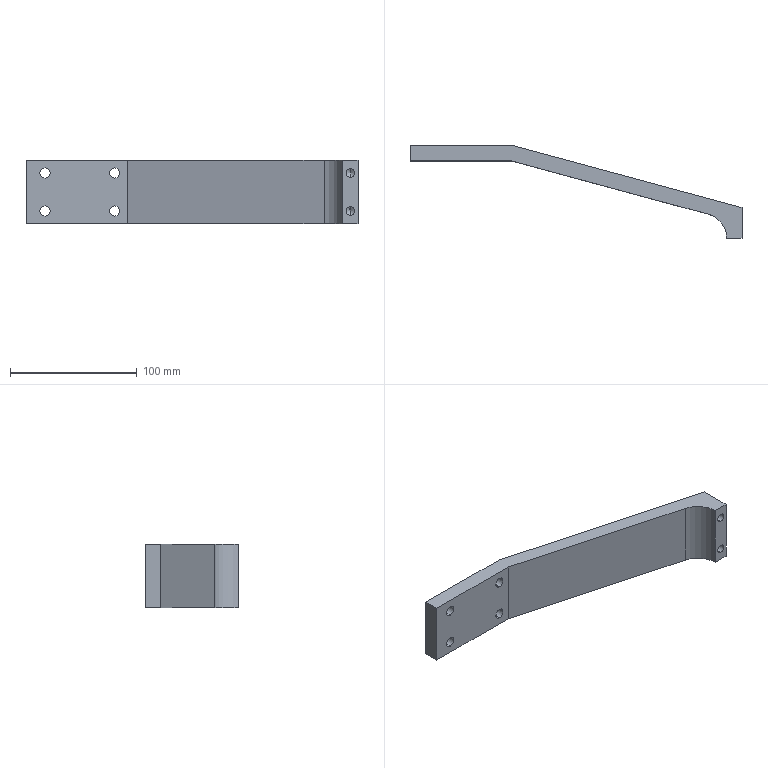Part | SolidWorks | features BaseBody 1 | 1 solid | 26 faces | box 262 x 73 x 50 mm | volume 167970 mm3 | cylinder 13 | plane 9 | cone 4 | commonest cylinder face diameters 8 x8 6.8 x4 40 x1
STEP:
#1=CARTESIAN_POINT('',(-260.,-92.,251.121));
#2=VERTEX_POINT('',#1);
#3=CARTESIAN_POINT('',(-260.,-92.,243.121));
#4=VERTEX_POINT('',#3);
#5=CARTESIAN_POINT('',(-260.,-92.,247.121));
#6=DIRECTION('',(0.,-1.,0.));
#7=DIRECTION('',(0.,0.,1.));
#8=AXIS2_PLACEMENT_3D('',#5,#6,#7);
#9=CIRCLE('',#8,4.);
#10=EDGE_CURVE('',#2,#4,#9,.T.);
#11=ORIENTED_EDGE('',*,*,#10,.T.);
#12=CARTESIAN_POINT('',(-260.,-80.,243.121));
#13=VERTEX_POINT('',#12);
#14=CARTESIAN_POINT('',(-260.,-153.,243.121));
#15=DIRECTION('',(0.,1.,0.));
#16=VECTOR('',#15,1000.);
#17=LINE('',#14,#16);
#18=EDGE_CURVE('',#4,#13,#17,.T.);
#19=ORIENTED_EDGE('',*,*,#18,.T.);
#20=CARTESIAN_POINT('',(-260.,-80.,251.121));
#21=VERTEX_POINT('',#20);
#22=CARTESIAN_POINT('',(-260.,-80.,247.121));
#23=DIRECTION('',(0.,1.,0.));
#24=DIRECTION('',(0.,0.,1.));
#25=AXIS2_PLACEMENT_3D('',#22,#23,#24);
#26=CIRCLE('',#25,4.);
#27=EDGE_CURVE('',#13,#21,#26,.T.);
#28=ORIENTED_EDGE('',*,*,#27,.T.);
#29=CARTESIAN_POINT('',(-260.,-153.,251.121));
#30=DIRECTION('',(0.,1.,0.));
#31=VECTOR('',#30,1000.);
#32=LINE('',#29,#31);
#33=EDGE_CURVE('',#2,#21,#32,.T.);
#34=ORIENTED_EDGE('',*,*,#33,.F.);
#35=EDGE_LOOP('',(#11,#19,#28,#34));
#36=FACE_OUTER_BOUND('',#35,.T.);
#37=CARTESIAN_POINT('',(-260.,-153.,247.121));
#38=DIRECTION('',(0.,1.,0.));
#39=DIRECTION('',(0.,0.,1.));
#40=AXIS2_PLACEMENT_3D('',#37,#38,#39);
#41=CYLINDRICAL_SURFACE('',#40,4.);
#42=ADVANCED_FACE('',(#36),#41,.F.);
#43=CARTESIAN_POINT('',(-260.,-92.,221.121));
#44=VERTEX_POINT('',#43);
#45=CARTESIAN_POINT('',(-260.,-92.,213.121));
#46=VERTEX_POINT('',#45);
#47=CARTESIAN_POINT('',(-260.,-92.,217.121));
#48=DIRECTION('',(0.,-1.,0.));
#49=DIRECTION('',(0.,0.,1.));
#50=AXIS2_PLACEMENT_3D('',#47,#48,#49);
#51=CIRCLE('',#50,4.);
#52=EDGE_CURVE('',#44,#46,#51,.T.);
#53=ORIENTED_EDGE('',*,*,#52,.T.);
#54=CARTESIAN_POINT('',(-260.,-80.,213.121));
#55=VERTEX_POINT('',#54);
#56=CARTESIAN_POINT('',(-260.,-153.,213.121));
#57=DIRECTION('',(0.,1.,0.));
#58=VECTOR('',#57,1000.);
#59=LINE('',#56,#58);
#60=EDGE_CURVE('',#46,#55,#59,.T.);
#61=ORIENTED_EDGE('',*,*,#60,.T.);
#62=CARTESIAN_POINT('',(-260.,-80.,221.121));
#63=VERTEX_POINT('',#62);
#64=CARTESIAN_POINT('',(-260.,-80.,217.121));
#65=DIRECTION('',(0.,1.,0.));
#66=DIRECTION('',(0.,0.,1.));
#67=AXIS2_PLACEMENT_3D('',#64,#65,#66);
#68=CIRCLE('',#67,4.);
#69=EDGE_CURVE('',#55,#63,#68,.T.);
#70=ORIENTED_EDGE('',*,*,#69,.T.);
#71=CARTESIAN_POINT('',(-260.,-153.,221.121));
#72=DIRECTION('',(0.,1.,0.));
#73=VECTOR('',#72,1000.);
#74=LINE('',#71,#73);
#75=EDGE_CURVE('',#44,#63,#74,.T.);
#76=ORIENTED_EDGE('',*,*,#75,.F.);
#77=EDGE_LOOP('',(#53,#61,#70,#76));
#78=FACE_OUTER_BOUND('',#77,.T.);
#79=CARTESIAN_POINT('',(-260.,-153.,217.121));
#80=DIRECTION('',(0.,1.,0.));
#81=DIRECTION('',(0.,0.,1.));
#82=AXIS2_PLACEMENT_3D('',#79,#80,#81);
#83=CYLINDRICAL_SURFACE('',#82,4.);
#84=ADVANCED_FACE('',(#78),#83,.F.);
#85=CARTESIAN_POINT('',(-315.,-92.,221.121));
#86=VERTEX_POINT('',#85);
#87=CARTESIAN_POINT('',(-315.,-92.,213.121));
#88=VERTEX_POINT('',#87);
#89=CARTESIAN_POINT('',(-315.,-92.,217.121));
#90=DIRECTION('',(0.,-1.,0.));
#91=DIRECTION('',(0.,0.,1.));
#92=AXIS2_PLACEMENT_3D('',#89,#90,#91);
#93=CIRCLE('',#92,4.);
#94=EDGE_CURVE('',#86,#88,#93,.T.);
#95=ORIENTED_EDGE('',*,*,#94,.T.);
#96=CARTESIAN_POINT('',(-315.,-80.,213.121));
#97=VERTEX_POINT('',#96);
#98=CARTESIAN_POINT('',(-315.,-153.,213.121));
#99=DIRECTION('',(0.,1.,0.));
#100=VECTOR('',#99,1000.);
#101=LINE('',#98,#100);
#102=EDGE_CURVE('',#88,#97,#101,.T.);
#103=ORIENTED_EDGE('',*,*,#102,.T.);
#104=CARTESIAN_POINT('',(-315.,-80.,221.121));
#105=VERTEX_POINT('',#104);
#106=CARTESIAN_POINT('',(-315.,-80.,217.121));
#107=DIRECTION('',(0.,1.,0.));
#108=DIRECTION('',(0.,0.,1.));
#109=AXIS2_PLACEMENT_3D('',#106,#107,#108);
#110=CIRCLE('',#109,4.);
#111=EDGE_CURVE('',#97,#105,#110,.T.);
#112=ORIENTED_EDGE('',*,*,#111,.T.);
#113=CARTESIAN_POINT('',(-315.,-153.,221.121));
#114=DIRECTION('',(0.,1.,0.));
#115=VECTOR('',#114,1000.);
#116=LINE('',#113,#115);
#117=EDGE_CURVE('',#86,#105,#116,.T.);
#118=ORIENTED_EDGE('',*,*,#117,.F.);
#119=EDGE_LOOP('',(#95,#103,#112,#118));
#120=FACE_OUTER_BOUND('',#119,.T.);
#121=CARTESIAN_POINT('',(-315.,-153.,217.121));
#122=DIRECTION('',(0.,1.,0.));
#123=DIRECTION('',(0.,0.,1.));
#124=AXIS2_PLACEMENT_3D('',#121,#122,#123);
#125=CYLINDRICAL_SURFACE('',#124,4.);
#126=ADVANCED_FACE('',(#120),#125,.F.);
#127=CARTESIAN_POINT('',(-315.,-92.,251.121));
#128=VERTEX_POINT('',#127);
#129=CARTESIAN_POINT('',(-315.,-92.,243.121));
#130=VERTEX_POINT('',#129);
#131=CARTESIAN_POINT('',(-315.,-92.,247.121));
#132=DIRECTION('',(0.,-1.,0.));
#133=DIRECTION('',(0.,0.,1.));
#134=AXIS2_PLACEMENT_3D('',#131,#132,#133);
#135=CIRCLE('',#134,4.);
#136=EDGE_CURVE('',#128,#130,#135,.T.);
#137=ORIENTED_EDGE('',*,*,#136,.T.);
#138=CARTESIAN_POINT('',(-315.,-80.,243.121));
#139=VERTEX_POINT('',#138);
#140=CARTESIAN_POINT('',(-315.,-153.,243.121));
#141=DIRECTION('',(0.,1.,0.));
#142=VECTOR('',#141,1000.);
#143=LINE('',#140,#142);
#144=EDGE_CURVE('',#130,#139,#143,.T.);
#145=ORIENTED_EDGE('',*,*,#144,.T.);
#146=CARTESIAN_POINT('',(-315.,-80.,251.121));
#147=VERTEX_POINT('',#146);
#148=CARTESIAN_POINT('',(-315.,-80.,247.121));
#149=DIRECTION('',(0.,1.,0.));
#150=DIRECTION('',(0.,0.,1.));
#151=AXIS2_PLACEMENT_3D('',#148,#149,#150);
#152=CIRCLE('',#151,4.);
#153=EDGE_CURVE('',#139,#147,#152,.T.);
#154=ORIENTED_EDGE('',*,*,#153,.T.);
#155=CARTESIAN_POINT('',(-315.,-153.,251.121));
#156=DIRECTION('',(0.,1.,0.));
#157=VECTOR('',#156,1000.);
#158=LINE('',#155,#157);
#159=EDGE_CURVE('',#128,#147,#158,.T.);
#160=ORIENTED_EDGE('',*,*,#159,.F.);
#161=EDGE_LOOP('',(#137,#145,#154,#160));
#162=FACE_OUTER_BOUND('',#161,.T.);
#163=CARTESIAN_POINT('',(-315.,-153.,247.121));
#164=DIRECTION('',(0.,1.,0.));
#165=DIRECTION('',(0.,0.,1.));
#166=AXIS2_PLACEMENT_3D('',#163,#164,#165);
#167=CYLINDRICAL_SURFACE('',#166,4.);
#168=ADVANCED_FACE('',(#162),#167,.F.);
#169=CARTESIAN_POINT('',(-74.,-140.,220.521));
#170=VERTEX_POINT('',#169);
#171=CARTESIAN_POINT('',(-74.,-140.,213.721));
#172=VERTEX_POINT('',#171);
#173=CARTESIAN_POINT('',(-74.,-140.,217.121));
#174=DIRECTION('',(0.,-1.,0.));
#175=DIRECTION('',(0.,0.,-1.));
#176=AXIS2_PLACEMENT_3D('',#173,#174,#175);
#177=CIRCLE('',#176,3.4);
#178=EDGE_CURVE('',#170,#172,#177,.T.);
#179=ORIENTED_EDGE('',*,*,#178,.F.);
#180=CARTESIAN_POINT('',(-74.,-153.,220.521));
#181=VERTEX_POINT('',#180);
#182=CARTESIAN_POINT('',(-74.,-153.,220.521));
#183=DIRECTION('',(0.,-1.,0.));
#184=VECTOR('',#183,1000.);
#185=LINE('',#182,#184);
#186=EDGE_CURVE('',#170,#181,#185,.T.);
#187=ORIENTED_EDGE('',*,*,#186,.T.);
#188=CARTESIAN_POINT('',(-74.,-153.,213.721));
#189=VERTEX_POINT('',#188);
#190=CARTESIAN_POINT('',(-74.,-153.,217.121));
#191=DIRECTION('',(0.,-1.,0.));
#192=DIRECTION('',(0.,0.,-1.));
#193=AXIS2_PLACEMENT_3D('',#190,#191,#192);
#194=CIRCLE('',#193,3.4);
#195=EDGE_CURVE('',#181,#189,#194,.T.);
#196=ORIENTED_EDGE('',*,*,#195,.T.);
#197=CARTESIAN_POINT('',(-74.,-153.,213.721));
#198=DIRECTION('',(0.,-1.,0.));
#199=VECTOR('',#198,1000.);
#200=LINE('',#197,#199);
#201=EDGE_CURVE('',#172,#189,#200,.T.);
#202=ORIENTED_EDGE('',*,*,#201,.F.);
#203=EDGE_LOOP('',(#179,#187,#196,#202));
#204=FACE_OUTER_BOUND('',#203,.T.);
#205=CARTESIAN_POINT('',(-74.,-153.,217.121));
#206=DIRECTION('',(0.,-1.,0.));
#207=DIRECTION('',(0.,0.,-1.));
#208=AXIS2_PLACEMENT_3D('',#205,#206,#207);
#209=CYLINDRICAL_SURFACE('',#208,3.4);
#210=ADVANCED_FACE('',(#204),#209,.F.);
#211=CARTESIAN_POINT('',(-74.,-140.,250.521));
#212=VERTEX_POINT('',#211);
#213=CARTESIAN_POINT('',(-74.,-140.,243.721));
#214=VERTEX_POINT('',#213);
#215=CARTESIAN_POINT('',(-74.,-140.,247.121));
#216=DIRECTION('',(0.,-1.,0.));
#217=DIRECTION('',(0.,0.,-1.));
#218=AXIS2_PLACEMENT_3D('',#215,#216,#217);
#219=CIRCLE('',#218,3.4);
#220=EDGE_CURVE('',#212,#214,#219,.T.);
#221=ORIENTED_EDGE('',*,*,#220,.F.);
#222=CARTESIAN_POINT('',(-74.,-153.,250.521));
#223=VERTEX_POINT('',#222);
#224=CARTESIAN_POINT('',(-74.,-153.,250.521));
#225=DIRECTION('',(0.,-1.,0.));
#226=VECTOR('',#225,1000.);
#227=LINE('',#224,#226);
#228=EDGE_CURVE('',#212,#223,#227,.T.);
#229=ORIENTED_EDGE('',*,*,#228,.T.);
#230=CARTESIAN_POINT('',(-74.,-153.,243.721));
#231=VERTEX_POINT('',#230);
#232=CARTESIAN_POINT('',(-74.,-153.,247.121));
#233=DIRECTION('',(0.,-1.,0.));
#234=DIRECTION('',(0.,0.,-1.));
#235=AXIS2_PLACEMENT_3D('',#232,#233,#234);
#236=CIRCLE('',#235,3.4);
#237=EDGE_CURVE('',#223,#231,#236,.T.);
#238=ORIENTED_EDGE('',*,*,#237,.T.);
#239=CARTESIAN_POINT('',(-74.,-153.,243.721));
#240=DIRECTION('',(0.,-1.,0.));
#241=VECTOR('',#240,1000.);
#242=LINE('',#239,#241);
#243=EDGE_CURVE('',#214,#231,#242,.T.);
#244=ORIENTED_EDGE('',*,*,#243,.F.);
#245=EDGE_LOOP('',(#221,#229,#238,#244));
#246=FACE_OUTER_BOUND('',#245,.T.);
#247=CARTESIAN_POINT('',(-74.,-153.,247.121));
#248=DIRECTION('',(0.,-1.,0.));
#249=DIRECTION('',(0.,0.,-1.));
#250=AXIS2_PLACEMENT_3D('',#247,#248,#249);
#251=CYLINDRICAL_SURFACE('',#250,3.4);
#252=ADVANCED_FACE('',(#246),#251,.F.);
#253=CARTESIAN_POINT('',(-74.,-137.957,217.121));
#254=VERTEX_POINT('',#253);
#255=CARTESIAN_POINT('',(-74.,-140.,213.721));
#256=DIRECTION('',(0.,-0.515,-0.8572));
#257=VECTOR('',#256,1000.);
#258=LINE('',#255,#257);
#259=EDGE_CURVE('',#254,#172,#258,.T.);
#260=ORIENTED_EDGE('',*,*,#259,.F.);
#261=CARTESIAN_POINT('',(-74.,-140.,220.521));
#262=DIRECTION('',(0.,-0.515,0.8572));
#263=VECTOR('',#262,1000.);
#264=LINE('',#261,#263);
#265=EDGE_CURVE('',#254,#170,#264,.T.);
#266=ORIENTED_EDGE('',*,*,#265,.T.);
#267=ORIENTED_EDGE('',*,*,#178,.T.);
#268=EDGE_LOOP('',(#260,#266,#267));
#269=FACE_OUTER_BOUND('',#268,.T.);
#270=CARTESIAN_POINT('',(-74.,-140.,217.121));
#271=DIRECTION('',(0.,-1.,0.));
#272=DIRECTION('',(0.,0.,-1.));
#273=AXIS2_PLACEMENT_3D('',#270,#271,#272);
#274=CONICAL_SURFACE('',#273,3.4,1.03);
#275=ADVANCED_FACE('',(#269),#274,.F.);
#276=CARTESIAN_POINT('',(-74.,-137.957,247.121));
#277=VERTEX_POINT('',#276);
#278=CARTESIAN_POINT('',(-74.,-140.,243.721));
#279=DIRECTION('',(0.,-0.515,-0.8572));
#280=VECTOR('',#279,1000.);
#281=LINE('',#278,#280);
#282=EDGE_CURVE('',#277,#214,#281,.T.);
#283=ORIENTED_EDGE('',*,*,#282,.F.);
#284=CARTESIAN_POINT('',(-74.,-140.,250.521));
#285=DIRECTION('',(0.,-0.515,0.8572));
#286=VECTOR('',#285,1000.);
#287=LINE('',#284,#286);
#288=EDGE_CURVE('',#277,#212,#287,.T.);
#289=ORIENTED_EDGE('',*,*,#288,.T.);
#290=ORIENTED_EDGE('',*,*,#220,.T.);
#291=EDGE_LOOP('',(#283,#289,#290));
#292=FACE_OUTER_BOUND('',#291,.T.);
#293=CARTESIAN_POINT('',(-74.,-140.,247.121));
#294=DIRECTION('',(0.,-1.,0.));
#295=DIRECTION('',(0.,0.,-1.));
#296=AXIS2_PLACEMENT_3D('',#293,#294,#295);
#297=CONICAL_SURFACE('',#296,3.4,1.03);
#298=ADVANCED_FACE('',(#292),#297,.F.);
#299=CARTESIAN_POINT('',(-248.405,-80.,257.121));
#300=VERTEX_POINT('',#299);
#301=CARTESIAN_POINT('',(-248.405,-80.,207.121));
#302=VERTEX_POINT('',#301);
#303=CARTESIAN_POINT('',(-248.405,-80.,257.121));
#304=DIRECTION('',(0.,0.,-1.));
#305=VECTOR('',#304,1000.);
#306=LINE('',#303,#305);
#307=EDGE_CURVE('',#300,#302,#306,.T.);
#308=ORIENTED_EDGE('',*,*,#307,.F.);
#309=CARTESIAN_POINT('',(-68.,-128.816,257.121));
#310=VERTEX_POINT('',#309);
#311=CARTESIAN_POINT('',(-68.,-128.816,257.121));
#312=DIRECTION('',(-0.9653,0.2612,0.));
#313=VECTOR('',#312,1000.);
#314=LINE('',#311,#313);
#315=EDGE_CURVE('',#310,#300,#314,.T.);
#316=ORIENTED_EDGE('',*,*,#315,.F.);
#317=CARTESIAN_POINT('',(-68.,-128.816,207.121));
#318=VERTEX_POINT('',#317);
#319=CARTESIAN_POINT('',(-68.,-128.816,257.121));
#320=DIRECTION('',(0.,0.,1.));
#321=VECTOR('',#320,1000.);
#322=LINE('',#319,#321);
#323=EDGE_CURVE('',#318,#310,#322,.T.);
#324=ORIENTED_EDGE('',*,*,#323,.F.);
#325=CARTESIAN_POINT('',(-68.,-128.816,207.121));
#326=DIRECTION('',(0.9653,-0.2612,0.));
#327=VECTOR('',#326,1000.);
#328=LINE('',#325,#327);
#329=EDGE_CURVE('',#302,#318,#328,.T.);
#330=ORIENTED_EDGE('',*,*,#329,.F.);
#331=EDGE_LOOP('',(#308,#316,#324,#330));
#332=FACE_OUTER_BOUND('',#331,.T.);
#333=CARTESIAN_POINT('',(-68.,-128.816,257.121));
#334=DIRECTION('',(-0.2612,-0.9653,0.));
#335=DIRECTION('',(0.9653,-0.2612,0.));
#336=AXIS2_PLACEMENT_3D('',#333,#334,#335);
#337=PLANE('',#336);
#338=ADVANCED_FACE('',(#332),#337,.F.);
#339=CARTESIAN_POINT('',(-94.774,-134.002,207.121));
#340=VERTEX_POINT('',#339);
#341=CARTESIAN_POINT('',(-80.,-153.,207.121));
#342=VERTEX_POINT('',#341);
#343=CARTESIAN_POINT('',(-99.998,-153.308,207.121));
#344=DIRECTION('',(0.,0.,-1.));
#345=DIRECTION('',(1.,0.,0.));
#346=AXIS2_PLACEMENT_3D('',#343,#344,#345);
#347=CIRCLE('',#346,20.);
#348=EDGE_CURVE('',#340,#342,#347,.T.);
#349=ORIENTED_EDGE('',*,*,#348,.F.);
#350=CARTESIAN_POINT('',(-250.,-92.,207.121));
#351=VERTEX_POINT('',#350);
#352=CARTESIAN_POINT('',(-250.,-92.,207.121));
#353=DIRECTION('',(0.9653,-0.2612,0.));
#354=VECTOR('',#353,1000.);
#355=LINE('',#352,#354);
#356=EDGE_CURVE('',#351,#340,#355,.T.);
#357=ORIENTED_EDGE('',*,*,#356,.F.);
#358=CARTESIAN_POINT('',(-330.,-92.,207.121));
#359=VERTEX_POINT('',#358);
#360=CARTESIAN_POINT('',(-68.,-92.,207.121));
#361=DIRECTION('',(1.,0.,0.));
#362=VECTOR('',#361,1000.);
#363=LINE('',#360,#362);
#364=EDGE_CURVE('',#359,#351,#363,.T.);
#365=ORIENTED_EDGE('',*,*,#364,.F.);
#366=CARTESIAN_POINT('',(-330.,-80.,207.121));
#367=VERTEX_POINT('',#366);
#368=CARTESIAN_POINT('',(-330.,-108.6,207.121));
#369=DIRECTION('',(0.,-1.,0.));
#370=VECTOR('',#369,1000.);
#371=LINE('',#368,#370);
#372=EDGE_CURVE('',#367,#359,#371,.T.);
#373=ORIENTED_EDGE('',*,*,#372,.F.);
#374=CARTESIAN_POINT('',(-68.,-80.,207.121));
#375=DIRECTION('',(-1.,0.,0.));
#376=VECTOR('',#375,1000.);
#377=LINE('',#374,#376);
#378=EDGE_CURVE('',#302,#367,#377,.T.);
#379=ORIENTED_EDGE('',*,*,#378,.F.);
#380=ORIENTED_EDGE('',*,*,#329,.T.);
#381=CARTESIAN_POINT('',(-68.,-153.,207.121));
#382=VERTEX_POINT('',#381);
#383=CARTESIAN_POINT('',(-68.,-108.6,207.121));
#384=DIRECTION('',(0.,1.,0.));
#385=VECTOR('',#384,1000.);
#386=LINE('',#383,#385);
#387=EDGE_CURVE('',#382,#318,#386,.T.);
#388=ORIENTED_EDGE('',*,*,#387,.F.);
#389=CARTESIAN_POINT('',(-68.,-153.,207.121));
#390=DIRECTION('',(1.,0.,0.));
#391=VECTOR('',#390,1000.);
#392=LINE('',#389,#391);
#393=EDGE_CURVE('',#342,#382,#392,.T.);
#394=ORIENTED_EDGE('',*,*,#393,.F.);
#395=EDGE_LOOP('',(#349,#357,#365,#373,#379,#380,#388,#394));
#396=FACE_OUTER_BOUND('',#395,.T.);
#397=CARTESIAN_POINT('',(-68.,-108.6,207.121));
#398=DIRECTION('',(0.,0.,1.));
#399=DIRECTION('',(1.,0.,0.));
#400=AXIS2_PLACEMENT_3D('',#397,#398,#399);
#401=PLANE('',#400);
#402=ADVANCED_FACE('',(#396),#401,.F.);
#403=CARTESIAN_POINT('',(-330.,-80.,257.121));
#404=VERTEX_POINT('',#403);
#405=CARTESIAN_POINT('',(-330.,-80.,257.121));
#406=DIRECTION('',(0.,0.,-1.));
#407=VECTOR('',#406,1000.);
#408=LINE('',#405,#407);
#409=EDGE_CURVE('',#404,#367,#408,.T.);
#410=ORIENTED_EDGE('',*,*,#409,.F.);
#411=CARTESIAN_POINT('',(-248.405,-80.,257.121));
#412=DIRECTION('',(-1.,0.,0.));
#413=VECTOR('',#412,1000.);
#414=LINE('',#411,#413);
#415=EDGE_CURVE('',#300,#404,#414,.T.);
#416=ORIENTED_EDGE('',*,*,#415,.F.);
#417=ORIENTED_EDGE('',*,*,#307,.T.);
#418=ORIENTED_EDGE('',*,*,#378,.T.);
#419=EDGE_LOOP('',(#410,#416,#417,#418));
#420=FACE_OUTER_BOUND('',#419,.T.);
#421=CARTESIAN_POINT('',(-260.,-80.,247.121));
#422=DIRECTION('',(0.,1.,0.));
#423=DIRECTION('',(0.,0.,1.));
#424=AXIS2_PLACEMENT_3D('',#421,#422,#423);
#425=CIRCLE('',#424,4.);
#426=EDGE_CURVE('',#21,#13,#425,.T.);
#427=ORIENTED_EDGE('',*,*,#426,.F.);
#428=ORIENTED_EDGE('',*,*,#27,.F.);
#429=EDGE_LOOP('',(#427,#428));
#430=FACE_BOUND('',#429,.T.);
#431=CARTESIAN_POINT('',(-260.,-80.,217.121));
#432=DIRECTION('',(0.,1.,0.));
#433=DIRECTION('',(0.,0.,1.));
#434=AXIS2_PLACEMENT_3D('',#431,#432,#433);
#435=CIRCLE('',#434,4.);
#436=EDGE_CURVE('',#63,#55,#435,.T.);
#437=ORIENTED_EDGE('',*,*,#436,.F.);
#438=ORIENTED_EDGE('',*,*,#69,.F.);
#439=EDGE_LOOP('',(#437,#438));
#440=FACE_BOUND('',#439,.T.);
#441=CARTESIAN_POINT('',(-315.,-80.,217.121));
#442=DIRECTION('',(0.,1.,0.));
#443=DIRECTION('',(0.,0.,1.));
#444=AXIS2_PLACEMENT_3D('',#441,#442,#443);
#445=CIRCLE('',#444,4.);
#446=EDGE_CURVE('',#105,#97,#445,.T.);
#447=ORIENTED_EDGE('',*,*,#446,.F.);
#448=ORIENTED_EDGE('',*,*,#111,.F.);
#449=EDGE_LOOP('',(#447,#448));
#450=FACE_BOUND('',#449,.T.);
#451=CARTESIAN_POINT('',(-315.,-80.,247.121));
#452=DIRECTION('',(0.,1.,0.));
#453=DIRECTION('',(0.,0.,1.));
#454=AXIS2_PLACEMENT_3D('',#451,#452,#453);
#455=CIRCLE('',#454,4.);
#456=EDGE_CURVE('',#147,#139,#455,.T.);
#457=ORIENTED_EDGE('',*,*,#456,.F.);
#458=ORIENTED_EDGE('',*,*,#153,.F.);
#459=EDGE_LOOP('',(#457,#458));
#460=FACE_BOUND('',#459,.T.);
#461=CARTESIAN_POINT('',(-248.405,-80.,257.121));
#462=DIRECTION('',(0.,-1.,0.));
#463=DIRECTION('',(0.,0.,-1.));
#464=AXIS2_PLACEMENT_3D('',#461,#462,#463);
#465=PLANE('',#464);
#466=ADVANCED_FACE('',(#420,#430,#440,#450,#460),#465,.F.);
#467=CARTESIAN_POINT('',(-250.,-92.,257.121));
#468=VERTEX_POINT('',#467);
#469=CARTESIAN_POINT('',(-94.774,-134.002,257.121));
#470=VERTEX_POINT('',#469);
#471=CARTESIAN_POINT('',(-250.,-92.,257.121));
#472=DIRECTION('',(0.9653,-0.2612,0.));
#473=VECTOR('',#472,1000.);
#474=LINE('',#471,#473);
#475=EDGE_CURVE('',#468,#470,#474,.T.);
#476=ORIENTED_EDGE('',*,*,#475,.T.);
#477=CARTESIAN_POINT('',(-80.,-153.,257.121));
#478=VERTEX_POINT('',#477);
#479=CARTESIAN_POINT('',(-99.998,-153.308,257.121));
#480=DIRECTION('',(0.,0.,-1.));
#481=DIRECTION('',(1.,0.,0.));
#482=AXIS2_PLACEMENT_3D('',#479,#480,#481);
#483=CIRCLE('',#482,20.);
#484=EDGE_CURVE('',#470,#478,#483,.T.);
#485=ORIENTED_EDGE('',*,*,#484,.T.);
#486=CARTESIAN_POINT('',(-68.,-153.,257.121));
#487=VERTEX_POINT('',#486);
#488=CARTESIAN_POINT('',(-68.,-153.,257.121));
#489=DIRECTION('',(1.,0.,0.));
#490=VECTOR('',#489,1000.);
#491=LINE('',#488,#490);
#492=EDGE_CURVE('',#478,#487,#491,.T.);
#493=ORIENTED_EDGE('',*,*,#492,.T.);
#494=CARTESIAN_POINT('',(-68.,-108.6,257.121));
#495=DIRECTION('',(0.,1.,0.));
#496=VECTOR('',#495,1000.);
#497=LINE('',#494,#496);
#498=EDGE_CURVE('',#487,#310,#497,.T.);
#499=ORIENTED_EDGE('',*,*,#498,.T.);
#500=ORIENTED_EDGE('',*,*,#315,.T.);
#501=ORIENTED_EDGE('',*,*,#415,.T.);
#502=CARTESIAN_POINT('',(-330.,-92.,257.121));
#503=VERTEX_POINT('',#502);
#504=CARTESIAN_POINT('',(-330.,-108.6,257.121));
#505=DIRECTION('',(0.,-1.,0.));
#506=VECTOR('',#505,1000.);
#507=LINE('',#504,#506);
#508=EDGE_CURVE('',#404,#503,#507,.T.);
#509=ORIENTED_EDGE('',*,*,#508,.T.);
#510=CARTESIAN_POINT('',(-68.,-92.,257.121));
#511=DIRECTION('',(1.,0.,0.));
#512=VECTOR('',#511,1000.);
#513=LINE('',#510,#512);
#514=EDGE_CURVE('',#503,#468,#513,.T.);
#515=ORIENTED_EDGE('',*,*,#514,.T.);
#516=EDGE_LOOP('',(#476,#485,#493,#499,#500,#501,#509,#515));
#517=FACE_OUTER_BOUND('',#516,.T.);
#518=CARTESIAN_POINT('',(-68.,-108.6,257.121));
#519=DIRECTION('',(0.,0.,1.));
#520=DIRECTION('',(1.,0.,0.));
#521=AXIS2_PLACEMENT_3D('',#518,#519,#520);
#522=PLANE('',#521);
#523=ADVANCED_FACE('',(#517),#522,.T.);
#524=ORIENTED_EDGE('',*,*,#323,.T.);
#525=ORIENTED_EDGE('',*,*,#498,.F.);
#526=CARTESIAN_POINT('',(-68.,-153.,257.121));
#527=DIRECTION('',(0.,0.,1.));
#528=VECTOR('',#527,1000.);
#529=LINE('',#526,#528);
#530=EDGE_CURVE('',#382,#487,#529,.T.);
#531=ORIENTED_EDGE('',*,*,#530,.F.);
#532=ORIENTED_EDGE('',*,*,#387,.T.);
#533=EDGE_LOOP('',(#524,#525,#531,#532));
#534=FACE_OUTER_BOUND('',#533,.T.);
#535=CARTESIAN_POINT('',(-68.,-153.,257.121));
#536=DIRECTION('',(-1.,0.,0.));
#537=DIRECTION('',(0.,0.,1.));
#538=AXIS2_PLACEMENT_3D('',#535,#536,#537);
#539=PLANE('',#538);
#540=ADVANCED_FACE('',(#534),#539,.F.);
#541=ORIENTED_EDGE('',*,*,#530,.T.);
#542=ORIENTED_EDGE('',*,*,#492,.F.);
#543=CARTESIAN_POINT('',(-80.,-153.,257.121));
#544=DIRECTION('',(0.,0.,1.));
#545=VECTOR('',#544,1000.);
#546=LINE('',#543,#545);
#547=EDGE_CURVE('',#342,#478,#546,.T.);
#548=ORIENTED_EDGE('',*,*,#547,.F.);
#549=ORIENTED_EDGE('',*,*,#393,.T.);
#550=EDGE_LOOP('',(#541,#542,#548,#549));
#551=FACE_OUTER_BOUND('',#550,.T.);
#552=CARTESIAN_POINT('',(-74.,-153.,217.121));
#553=DIRECTION('',(0.,-1.,0.));
#554=DIRECTION('',(0.,0.,-1.));
#555=AXIS2_PLACEMENT_3D('',#552,#553,#554);
#556=CIRCLE('',#555,3.4);
#557=EDGE_CURVE('',#189,#181,#556,.T.);
#558=ORIENTED_EDGE('',*,*,#557,.F.);
#559=ORIENTED_EDGE('',*,*,#195,.F.);
#560=EDGE_LOOP('',(#558,#559));
#561=FACE_BOUND('',#560,.T.);
#562=CARTESIAN_POINT('',(-74.,-153.,247.121));
#563=DIRECTION('',(0.,-1.,0.));
#564=DIRECTION('',(0.,0.,-1.));
#565=AXIS2_PLACEMENT_3D('',#562,#563,#564);
#566=CIRCLE('',#565,3.4);
#567=EDGE_CURVE('',#231,#223,#566,.T.);
#568=ORIENTED_EDGE('',*,*,#567,.F.);
#569=ORIENTED_EDGE('',*,*,#237,.F.);
#570=EDGE_LOOP('',(#568,#569));
#571=FACE_BOUND('',#570,.T.);
#572=CARTESIAN_POINT('',(-80.,-153.,257.121));
#573=DIRECTION('',(0.,1.,0.));
#574=DIRECTION('',(0.,0.,1.));
#575=AXIS2_PLACEMENT_3D('',#572,#573,#574);
#576=PLANE('',#575);
#577=ADVANCED_FACE('',(#551,#561,#571),#576,.F.);
#578=CARTESIAN_POINT('',(-94.774,-134.002,257.121));
#579=DIRECTION('',(0.,0.,1.));
#580=VECTOR('',#579,1000.);
#581=LINE('',#578,#580);
#582=EDGE_CURVE('',#340,#470,#581,.T.);
#583=ORIENTED_EDGE('',*,*,#582,.F.);
#584=ORIENTED_EDGE('',*,*,#348,.T.);
#585=ORIENTED_EDGE('',*,*,#547,.T.);
#586=ORIENTED_EDGE('',*,*,#484,.F.);
#587=EDGE_LOOP('',(#583,#584,#585,#586));
#588=FACE_OUTER_BOUND('',#587,.T.);
#589=CARTESIAN_POINT('',(-99.998,-153.308,257.121));
#590=DIRECTION('',(0.,0.,1.));
#591=DIRECTION('',(1.,0.,0.));
#592=AXIS2_PLACEMENT_3D('',#589,#590,#591);
#593=CYLINDRICAL_SURFACE('',#592,20.);
#594=ADVANCED_FACE('',(#588),#593,.F.);
#595=ORIENTED_EDGE('',*,*,#582,.T.);
#596=ORIENTED_EDGE('',*,*,#475,.F.);
#597=CARTESIAN_POINT('',(-250.,-92.,257.121));
#598=DIRECTION('',(0.,0.,1.));
#599=VECTOR('',#598,1000.);
#600=LINE('',#597,#599);
#601=EDGE_CURVE('',#351,#468,#600,.T.);
#602=ORIENTED_EDGE('',*,*,#601,.F.);
#603=ORIENTED_EDGE('',*,*,#356,.T.);
#604=EDGE_LOOP('',(#595,#596,#602,#603));
#605=FACE_OUTER_BOUND('',#604,.T.);
#606=CARTESIAN_POINT('',(-80.,-138.,257.121));
#607=DIRECTION('',(0.2612,0.9653,0.));
#608=DIRECTION('',(-0.9653,0.2612,0.));
#609=AXIS2_PLACEMENT_3D('',#606,#607,#608);
#610=PLANE('',#609);
#611=ADVANCED_FACE('',(#605),#610,.F.);
#612=ORIENTED_EDGE('',*,*,#601,.T.);
#613=ORIENTED_EDGE('',*,*,#514,.F.);
#614=CARTESIAN_POINT('',(-330.,-92.,257.121));
#615=DIRECTION('',(0.,0.,1.));
#616=VECTOR('',#615,1000.);
#617=LINE('',#614,#616);
#618=EDGE_CURVE('',#359,#503,#617,.T.);
#619=ORIENTED_EDGE('',*,*,#618,.F.);
#620=ORIENTED_EDGE('',*,*,#364,.T.);
#621=EDGE_LOOP('',(#612,#613,#619,#620));
#622=FACE_OUTER_BOUND('',#621,.T.);
#623=ORIENTED_EDGE('',*,*,#10,.F.);
#624=CARTESIAN_POINT('',(-260.,-92.,247.121));
#625=DIRECTION('',(0.,-1.,0.));
#626=DIRECTION('',(0.,0.,1.));
#627=AXIS2_PLACEMENT_3D('',#624,#625,#626);
#628=CIRCLE('',#627,4.);
#629=EDGE_CURVE('',#4,#2,#628,.T.);
#630=ORIENTED_EDGE('',*,*,#629,.F.);
#631=EDGE_LOOP('',(#623,#630));
#632=FACE_BOUND('',#631,.T.);
#633=ORIENTED_EDGE('',*,*,#52,.F.);
#634=CARTESIAN_POINT('',(-260.,-92.,217.121));
#635=DIRECTION('',(0.,-1.,0.));
#636=DIRECTION('',(0.,0.,1.));
#637=AXIS2_PLACEMENT_3D('',#634,#635,#636);
#638=CIRCLE('',#637,4.);
#639=EDGE_CURVE('',#46,#44,#638,.T.);
#640=ORIENTED_EDGE('',*,*,#639,.F.);
#641=EDGE_LOOP('',(#633,#640));
#642=FACE_BOUND('',#641,.T.);
#643=ORIENTED_EDGE('',*,*,#94,.F.);
#644=CARTESIAN_POINT('',(-315.,-92.,217.121));
#645=DIRECTION('',(0.,-1.,0.));
#646=DIRECTION('',(0.,0.,1.));
#647=AXIS2_PLACEMENT_3D('',#644,#645,#646);
#648=CIRCLE('',#647,4.);
#649=EDGE_CURVE('',#88,#86,#648,.T.);
#650=ORIENTED_EDGE('',*,*,#649,.F.);
#651=EDGE_LOOP('',(#643,#650));
#652=FACE_BOUND('',#651,.T.);
#653=ORIENTED_EDGE('',*,*,#136,.F.);
#654=CARTESIAN_POINT('',(-315.,-92.,247.121));
#655=DIRECTION('',(0.,-1.,0.));
#656=DIRECTION('',(0.,0.,1.));
#657=AXIS2_PLACEMENT_3D('',#654,#655,#656);
#658=CIRCLE('',#657,4.);
#659=EDGE_CURVE('',#130,#128,#658,.T.);
#660=ORIENTED_EDGE('',*,*,#659,.F.);
#661=EDGE_LOOP('',(#653,#660));
#662=FACE_BOUND('',#661,.T.);
#663=CARTESIAN_POINT('',(-250.,-92.,257.121));
#664=DIRECTION('',(0.,1.,0.));
#665=DIRECTION('',(0.,0.,1.));
#666=AXIS2_PLACEMENT_3D('',#663,#664,#665);
#667=PLANE('',#666);
#668=ADVANCED_FACE('',(#622,#632,#642,#652,#662),#667,.F.);
#669=ORIENTED_EDGE('',*,*,#618,.T.);
#670=ORIENTED_EDGE('',*,*,#508,.F.);
#671=ORIENTED_EDGE('',*,*,#409,.T.);
#672=ORIENTED_EDGE('',*,*,#372,.T.);
#673=EDGE_LOOP('',(#669,#670,#671,#672));
#674=FACE_OUTER_BOUND('',#673,.T.);
#675=CARTESIAN_POINT('',(-330.,-80.,257.121));
#676=DIRECTION('',(1.,0.,0.));
#677=DIRECTION('',(0.,0.,-1.));
#678=AXIS2_PLACEMENT_3D('',#675,#676,#677);
#679=PLANE('',#678);
#680=ADVANCED_FACE('',(#674),#679,.F.);
#681=ORIENTED_EDGE('',*,*,#18,.F.);
#682=ORIENTED_EDGE('',*,*,#629,.T.);
#683=ORIENTED_EDGE('',*,*,#33,.T.);
#684=ORIENTED_EDGE('',*,*,#426,.T.);
#685=EDGE_LOOP('',(#681,#682,#683,#684));
#686=FACE_OUTER_BOUND('',#685,.T.);
#687=CARTESIAN_POINT('',(-260.,-153.,247.121));
#688=DIRECTION('',(0.,1.,0.));
#689=DIRECTION('',(0.,0.,1.));
#690=AXIS2_PLACEMENT_3D('',#687,#688,#689);
#691=CYLINDRICAL_SURFACE('',#690,4.);
#692=ADVANCED_FACE('',(#686),#691,.F.);
#693=ORIENTED_EDGE('',*,*,#60,.F.);
#694=ORIENTED_EDGE('',*,*,#639,.T.);
#695=ORIENTED_EDGE('',*,*,#75,.T.);
#696=ORIENTED_EDGE('',*,*,#436,.T.);
#697=EDGE_LOOP('',(#693,#694,#695,#696));
#698=FACE_OUTER_BOUND('',#697,.T.);
#699=CARTESIAN_POINT('',(-260.,-153.,217.121));
#700=DIRECTION('',(0.,1.,0.));
#701=DIRECTION('',(0.,0.,1.));
#702=AXIS2_PLACEMENT_3D('',#699,#700,#701);
#703=CYLINDRICAL_SURFACE('',#702,4.);
#704=ADVANCED_FACE('',(#698),#703,.F.);
#705=ORIENTED_EDGE('',*,*,#102,.F.);
#706=ORIENTED_EDGE('',*,*,#649,.T.);
#707=ORIENTED_EDGE('',*,*,#117,.T.);
#708=ORIENTED_EDGE('',*,*,#446,.T.);
#709=EDGE_LOOP('',(#705,#706,#707,#708));
#710=FACE_OUTER_BOUND('',#709,.T.);
#711=CARTESIAN_POINT('',(-315.,-153.,217.121));
#712=DIRECTION('',(0.,1.,0.));
#713=DIRECTION('',(0.,0.,1.));
#714=AXIS2_PLACEMENT_3D('',#711,#712,#713);
#715=CYLINDRICAL_SURFACE('',#714,4.);
#716=ADVANCED_FACE('',(#710),#715,.F.);
#717=ORIENTED_EDGE('',*,*,#144,.F.);
#718=ORIENTED_EDGE('',*,*,#659,.T.);
#719=ORIENTED_EDGE('',*,*,#159,.T.);
#720=ORIENTED_EDGE('',*,*,#456,.T.);
#721=EDGE_LOOP('',(#717,#718,#719,#720));
#722=FACE_OUTER_BOUND('',#721,.T.);
#723=CARTESIAN_POINT('',(-315.,-153.,247.121));
#724=DIRECTION('',(0.,1.,0.));
#725=DIRECTION('',(0.,0.,1.));
#726=AXIS2_PLACEMENT_3D('',#723,#724,#725);
#727=CYLINDRICAL_SURFACE('',#726,4.);
#728=ADVANCED_FACE('',(#722),#727,.F.);
#729=ORIENTED_EDGE('',*,*,#186,.F.);
#730=CARTESIAN_POINT('',(-74.,-140.,217.121));
#731=DIRECTION('',(0.,-1.,0.));
#732=DIRECTION('',(0.,0.,-1.));
#733=AXIS2_PLACEMENT_3D('',#730,#731,#732);
#734=CIRCLE('',#733,3.4);
#735=EDGE_CURVE('',#172,#170,#734,.T.);
#736=ORIENTED_EDGE('',*,*,#735,.F.);
#737=ORIENTED_EDGE('',*,*,#201,.T.);
#738=ORIENTED_EDGE('',*,*,#557,.T.);
#739=EDGE_LOOP('',(#729,#736,#737,#738));
#740=FACE_OUTER_BOUND('',#739,.T.);
#741=CARTESIAN_POINT('',(-74.,-153.,217.121));
#742=DIRECTION('',(0.,-1.,0.));
#743=DIRECTION('',(0.,0.,-1.));
#744=AXIS2_PLACEMENT_3D('',#741,#742,#743);
#745=CYLINDRICAL_SURFACE('',#744,3.4);
#746=ADVANCED_FACE('',(#740),#745,.F.);
#747=ORIENTED_EDGE('',*,*,#228,.F.);
#748=CARTESIAN_POINT('',(-74.,-140.,247.121));
#749=DIRECTION('',(0.,-1.,0.));
#750=DIRECTION('',(0.,0.,-1.));
#751=AXIS2_PLACEMENT_3D('',#748,#749,#750);
#752=CIRCLE('',#751,3.4);
#753=EDGE_CURVE('',#214,#212,#752,.T.);
#754=ORIENTED_EDGE('',*,*,#753,.F.);
#755=ORIENTED_EDGE('',*,*,#243,.T.);
#756=ORIENTED_EDGE('',*,*,#567,.T.);
#757=EDGE_LOOP('',(#747,#754,#755,#756));
#758=FACE_OUTER_BOUND('',#757,.T.);
#759=CARTESIAN_POINT('',(-74.,-153.,247.121));
#760=DIRECTION('',(0.,-1.,0.));
#761=DIRECTION('',(0.,0.,-1.));
#762=AXIS2_PLACEMENT_3D('',#759,#760,#761);
#763=CYLINDRICAL_SURFACE('',#762,3.4);
#764=ADVANCED_FACE('',(#758),#763,.F.);
#765=ORIENTED_EDGE('',*,*,#265,.F.);
#766=ORIENTED_EDGE('',*,*,#259,.T.);
#767=ORIENTED_EDGE('',*,*,#735,.T.);
#768=EDGE_LOOP('',(#765,#766,#767));
#769=FACE_OUTER_BOUND('',#768,.T.);
#770=CARTESIAN_POINT('',(-74.,-140.,217.121));
#771=DIRECTION('',(0.,-1.,0.));
#772=DIRECTION('',(0.,0.,-1.));
#773=AXIS2_PLACEMENT_3D('',#770,#771,#772);
#774=CONICAL_SURFACE('',#773,3.4,1.03);
#775=ADVANCED_FACE('',(#769),#774,.F.);
#776=ORIENTED_EDGE('',*,*,#288,.F.);
#777=ORIENTED_EDGE('',*,*,#282,.T.);
#778=ORIENTED_EDGE('',*,*,#753,.T.);
#779=EDGE_LOOP('',(#776,#777,#778));
#780=FACE_OUTER_BOUND('',#779,.T.);
#781=CARTESIAN_POINT('',(-74.,-140.,247.121));
#782=DIRECTION('',(0.,-1.,0.));
#783=DIRECTION('',(0.,0.,-1.));
#784=AXIS2_PLACEMENT_3D('',#781,#782,#783);
#785=CONICAL_SURFACE('',#784,3.4,1.03);
#786=ADVANCED_FACE('',(#780),#785,.F.);
#787=CLOSED_SHELL('',(#42,#84,#126,#168,#210,#252,#275,#298,#338,#402,#466,#523,#540,#577,#594,#611,#668,#680,#692,#704,#716,#728,#746,#764,#775,#786));
#788=MANIFOLD_SOLID_BREP('',#787);
#789=CARTESIAN_POINT('',(0.,0.,0.));
#790=DIRECTION('',(0.,0.,1.));
#791=DIRECTION('',(1.,0.,0.));
#792=AXIS2_PLACEMENT_3D('',#789,#790,#791);
#793=(LENGTH_UNIT()NAMED_UNIT(*)SI_UNIT(.MILLI.,.METRE.));
#794=UNCERTAINTY_MEASURE_WITH_UNIT(LENGTH_MEASURE(0.00001),#793,'','');
#795=(NAMED_UNIT(*)PLANE_ANGLE_UNIT()SI_UNIT($,.RADIAN.));
#796=(NAMED_UNIT(*)SI_UNIT($,.STERADIAN.)SOLID_ANGLE_UNIT());
#797=(GEOMETRIC_REPRESENTATION_CONTEXT(3)GLOBAL_UNCERTAINTY_ASSIGNED_CONTEXT((#794))GLOBAL_UNIT_ASSIGNED_CONTEXT((#793,#795,#796))REPRESENTATION_CONTEXT('',''));
#798=ADVANCED_BREP_SHAPE_REPRESENTATION('',(#788,#792),#797);